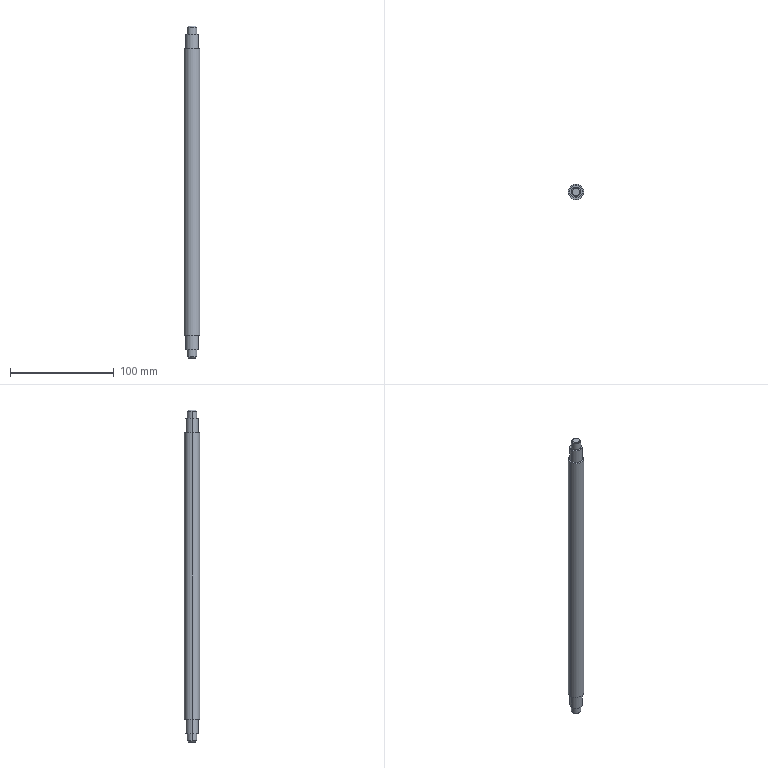Part | SolidWorks | features ICE 5, Chamfer 1, Extrusion 1, MirrorPattern 1 | 1 solid | 20 faces | box 15 x 15 x 320 mm | volume 52932 mm3 | cylinder 10 | plane 6 | cone 4 | commonest cylinder face diameters 9 x4 12 x4 15 x2
STEP:
#1=CARTESIAN_POINT('',(-3.5,0.,0.));
#2=VERTEX_POINT('',#1);
#3=CARTESIAN_POINT('',(3.5,0.,0.));
#4=VERTEX_POINT('',#3);
#5=CARTESIAN_POINT('',(0.,0.,0.));
#6=DIRECTION('',(0.,0.,-1.));
#7=DIRECTION('',(1.,0.,0.));
#8=AXIS2_PLACEMENT_3D('',#5,#6,#7);
#9=CIRCLE('',#8,3.5);
#10=EDGE_CURVE('',#2,#4,#9,.T.);
#11=ORIENTED_EDGE('',*,*,#10,.F.);
#12=CARTESIAN_POINT('',(-4.5,0.,1.));
#13=VERTEX_POINT('',#12);
#14=CARTESIAN_POINT('',(-4.5,0.,1.));
#15=DIRECTION('',(-0.7071,0.,0.7071));
#16=VECTOR('',#15,1000.);
#17=LINE('',#14,#16);
#18=EDGE_CURVE('',#2,#13,#17,.T.);
#19=ORIENTED_EDGE('',*,*,#18,.T.);
#20=CARTESIAN_POINT('',(4.5,0.,1.));
#21=VERTEX_POINT('',#20);
#22=CARTESIAN_POINT('',(0.,0.,1.));
#23=DIRECTION('',(0.,0.,1.));
#24=DIRECTION('',(1.,0.,0.));
#25=AXIS2_PLACEMENT_3D('',#22,#23,#24);
#26=CIRCLE('',#25,4.5);
#27=EDGE_CURVE('',#21,#13,#26,.T.);
#28=ORIENTED_EDGE('',*,*,#27,.F.);
#29=CARTESIAN_POINT('',(4.5,0.,1.));
#30=DIRECTION('',(0.7071,0.,0.7071));
#31=VECTOR('',#30,1000.);
#32=LINE('',#29,#31);
#33=EDGE_CURVE('',#4,#21,#32,.T.);
#34=ORIENTED_EDGE('',*,*,#33,.F.);
#35=EDGE_LOOP('',(#11,#19,#28,#34));
#36=FACE_OUTER_BOUND('',#35,.T.);
#37=CARTESIAN_POINT('',(0.,0.,1.));
#38=DIRECTION('',(0.,0.,1.));
#39=DIRECTION('',(1.,0.,0.));
#40=AXIS2_PLACEMENT_3D('',#37,#38,#39);
#41=CONICAL_SURFACE('',#40,4.5,0.7854);
#42=ADVANCED_FACE('',(#36),#41,.T.);
#43=CARTESIAN_POINT('',(3.5,0.,320.));
#44=VERTEX_POINT('',#43);
#45=CARTESIAN_POINT('',(-3.5,0.,320.));
#46=VERTEX_POINT('',#45);
#47=CARTESIAN_POINT('',(0.,0.,320.));
#48=DIRECTION('',(0.,0.,1.));
#49=DIRECTION('',(1.,0.,0.));
#50=AXIS2_PLACEMENT_3D('',#47,#48,#49);
#51=CIRCLE('',#50,3.5);
#52=EDGE_CURVE('',#44,#46,#51,.T.);
#53=ORIENTED_EDGE('',*,*,#52,.F.);
#54=CARTESIAN_POINT('',(4.5,0.,319.));
#55=VERTEX_POINT('',#54);
#56=CARTESIAN_POINT('',(3.5,0.,320.));
#57=DIRECTION('',(0.7071,0.,-0.7071));
#58=VECTOR('',#57,1000.);
#59=LINE('',#56,#58);
#60=EDGE_CURVE('',#44,#55,#59,.T.);
#61=ORIENTED_EDGE('',*,*,#60,.T.);
#62=CARTESIAN_POINT('',(-4.5,0.,319.));
#63=VERTEX_POINT('',#62);
#64=CARTESIAN_POINT('',(0.,0.,319.));
#65=DIRECTION('',(0.,0.,-1.));
#66=DIRECTION('',(1.,0.,0.));
#67=AXIS2_PLACEMENT_3D('',#64,#65,#66);
#68=CIRCLE('',#67,4.5);
#69=EDGE_CURVE('',#63,#55,#68,.T.);
#70=ORIENTED_EDGE('',*,*,#69,.F.);
#71=CARTESIAN_POINT('',(-3.5,0.,320.));
#72=DIRECTION('',(-0.7071,0.,-0.7071));
#73=VECTOR('',#72,1000.);
#74=LINE('',#71,#73);
#75=EDGE_CURVE('',#46,#63,#74,.T.);
#76=ORIENTED_EDGE('',*,*,#75,.F.);
#77=EDGE_LOOP('',(#53,#61,#70,#76));
#78=FACE_OUTER_BOUND('',#77,.T.);
#79=CARTESIAN_POINT('',(0.,0.,320.));
#80=DIRECTION('',(0.,0.,-1.));
#81=DIRECTION('',(-1.,0.,0.));
#82=AXIS2_PLACEMENT_3D('',#79,#80,#81);
#83=CONICAL_SURFACE('',#82,3.5,0.7854);
#84=ADVANCED_FACE('',(#78),#83,.T.);
#85=ORIENTED_EDGE('',*,*,#69,.T.);
#86=CARTESIAN_POINT('',(4.5,0.,312.));
#87=VERTEX_POINT('',#86);
#88=CARTESIAN_POINT('',(4.5,0.,320.));
#89=DIRECTION('',(0.,0.,-1.));
#90=VECTOR('',#89,1000.);
#91=LINE('',#88,#90);
#92=EDGE_CURVE('',#55,#87,#91,.T.);
#93=ORIENTED_EDGE('',*,*,#92,.T.);
#94=CARTESIAN_POINT('',(-4.5,0.,312.));
#95=VERTEX_POINT('',#94);
#96=CARTESIAN_POINT('',(0.,0.,312.));
#97=DIRECTION('',(0.,0.,1.));
#98=DIRECTION('',(1.,0.,0.));
#99=AXIS2_PLACEMENT_3D('',#96,#97,#98);
#100=CIRCLE('',#99,4.5);
#101=EDGE_CURVE('',#87,#95,#100,.T.);
#102=ORIENTED_EDGE('',*,*,#101,.T.);
#103=CARTESIAN_POINT('',(-4.5,0.,320.));
#104=DIRECTION('',(0.,0.,-1.));
#105=VECTOR('',#104,1000.);
#106=LINE('',#103,#105);
#107=EDGE_CURVE('',#63,#95,#106,.T.);
#108=ORIENTED_EDGE('',*,*,#107,.F.);
#109=EDGE_LOOP('',(#85,#93,#102,#108));
#110=FACE_OUTER_BOUND('',#109,.T.);
#111=CARTESIAN_POINT('',(0.,0.,320.));
#112=DIRECTION('',(0.,0.,-1.));
#113=DIRECTION('',(-1.,0.,0.));
#114=AXIS2_PLACEMENT_3D('',#111,#112,#113);
#115=CYLINDRICAL_SURFACE('',#114,4.5);
#116=ADVANCED_FACE('',(#110),#115,.T.);
#117=CARTESIAN_POINT('',(6.,0.,312.));
#118=VERTEX_POINT('',#117);
#119=CARTESIAN_POINT('',(-6.,0.,312.));
#120=VERTEX_POINT('',#119);
#121=CARTESIAN_POINT('',(0.,0.,312.));
#122=DIRECTION('',(0.,0.,1.));
#123=DIRECTION('',(1.,0.,0.));
#124=AXIS2_PLACEMENT_3D('',#121,#122,#123);
#125=CIRCLE('',#124,6.);
#126=EDGE_CURVE('',#118,#120,#125,.T.);
#127=ORIENTED_EDGE('',*,*,#126,.F.);
#128=CARTESIAN_POINT('',(6.,0.,298.));
#129=VERTEX_POINT('',#128);
#130=CARTESIAN_POINT('',(6.,0.,312.));
#131=DIRECTION('',(0.,0.,-1.));
#132=VECTOR('',#131,1000.);
#133=LINE('',#130,#132);
#134=EDGE_CURVE('',#118,#129,#133,.T.);
#135=ORIENTED_EDGE('',*,*,#134,.T.);
#136=CARTESIAN_POINT('',(-6.,0.,298.));
#137=VERTEX_POINT('',#136);
#138=CARTESIAN_POINT('',(0.,0.,298.));
#139=DIRECTION('',(0.,0.,1.));
#140=DIRECTION('',(1.,0.,0.));
#141=AXIS2_PLACEMENT_3D('',#138,#139,#140);
#142=CIRCLE('',#141,6.);
#143=EDGE_CURVE('',#129,#137,#142,.T.);
#144=ORIENTED_EDGE('',*,*,#143,.T.);
#145=CARTESIAN_POINT('',(-6.,0.,312.));
#146=DIRECTION('',(0.,0.,-1.));
#147=VECTOR('',#146,1000.);
#148=LINE('',#145,#147);
#149=EDGE_CURVE('',#120,#137,#148,.T.);
#150=ORIENTED_EDGE('',*,*,#149,.F.);
#151=EDGE_LOOP('',(#127,#135,#144,#150));
#152=FACE_OUTER_BOUND('',#151,.T.);
#153=CARTESIAN_POINT('',(0.,0.,312.));
#154=DIRECTION('',(0.,0.,-1.));
#155=DIRECTION('',(-1.,0.,0.));
#156=AXIS2_PLACEMENT_3D('',#153,#154,#155);
#157=CYLINDRICAL_SURFACE('',#156,6.);
#158=ADVANCED_FACE('',(#152),#157,.T.);
#159=CARTESIAN_POINT('',(7.5,0.,298.));
#160=VERTEX_POINT('',#159);
#161=CARTESIAN_POINT('',(-7.5,0.,298.));
#162=VERTEX_POINT('',#161);
#163=CARTESIAN_POINT('',(0.,0.,298.));
#164=DIRECTION('',(0.,0.,1.));
#165=DIRECTION('',(1.,0.,0.));
#166=AXIS2_PLACEMENT_3D('',#163,#164,#165);
#167=CIRCLE('',#166,7.5);
#168=EDGE_CURVE('',#160,#162,#167,.T.);
#169=ORIENTED_EDGE('',*,*,#168,.F.);
#170=CARTESIAN_POINT('',(7.5,0.,22.));
#171=VERTEX_POINT('',#170);
#172=CARTESIAN_POINT('',(7.5,0.,298.));
#173=DIRECTION('',(0.,0.,-1.));
#174=VECTOR('',#173,1000.);
#175=LINE('',#172,#174);
#176=EDGE_CURVE('',#160,#171,#175,.T.);
#177=ORIENTED_EDGE('',*,*,#176,.T.);
#178=CARTESIAN_POINT('',(-7.5,0.,22.));
#179=VERTEX_POINT('',#178);
#180=CARTESIAN_POINT('',(0.,0.,22.));
#181=DIRECTION('',(0.,0.,1.));
#182=DIRECTION('',(1.,0.,0.));
#183=AXIS2_PLACEMENT_3D('',#180,#181,#182);
#184=CIRCLE('',#183,7.5);
#185=EDGE_CURVE('',#171,#179,#184,.T.);
#186=ORIENTED_EDGE('',*,*,#185,.T.);
#187=CARTESIAN_POINT('',(-7.5,0.,298.));
#188=DIRECTION('',(0.,0.,-1.));
#189=VECTOR('',#188,1000.);
#190=LINE('',#187,#189);
#191=EDGE_CURVE('',#162,#179,#190,.T.);
#192=ORIENTED_EDGE('',*,*,#191,.F.);
#193=EDGE_LOOP('',(#169,#177,#186,#192));
#194=FACE_OUTER_BOUND('',#193,.T.);
#195=CARTESIAN_POINT('',(0.,0.,298.));
#196=DIRECTION('',(0.,0.,-1.));
#197=DIRECTION('',(-1.,0.,0.));
#198=AXIS2_PLACEMENT_3D('',#195,#196,#197);
#199=CYLINDRICAL_SURFACE('',#198,7.5);
#200=ADVANCED_FACE('',(#194),#199,.T.);
#201=CARTESIAN_POINT('',(6.,0.,22.));
#202=VERTEX_POINT('',#201);
#203=CARTESIAN_POINT('',(-6.,0.,22.));
#204=VERTEX_POINT('',#203);
#205=CARTESIAN_POINT('',(0.,0.,22.));
#206=DIRECTION('',(0.,0.,1.));
#207=DIRECTION('',(1.,0.,0.));
#208=AXIS2_PLACEMENT_3D('',#205,#206,#207);
#209=CIRCLE('',#208,6.);
#210=EDGE_CURVE('',#202,#204,#209,.T.);
#211=ORIENTED_EDGE('',*,*,#210,.F.);
#212=CARTESIAN_POINT('',(6.,0.,8.));
#213=VERTEX_POINT('',#212);
#214=CARTESIAN_POINT('',(6.,0.,22.));
#215=DIRECTION('',(0.,0.,-1.));
#216=VECTOR('',#215,1000.);
#217=LINE('',#214,#216);
#218=EDGE_CURVE('',#202,#213,#217,.T.);
#219=ORIENTED_EDGE('',*,*,#218,.T.);
#220=CARTESIAN_POINT('',(-6.,0.,8.));
#221=VERTEX_POINT('',#220);
#222=CARTESIAN_POINT('',(0.,0.,8.));
#223=DIRECTION('',(0.,0.,1.));
#224=DIRECTION('',(1.,0.,0.));
#225=AXIS2_PLACEMENT_3D('',#222,#223,#224);
#226=CIRCLE('',#225,6.);
#227=EDGE_CURVE('',#213,#221,#226,.T.);
#228=ORIENTED_EDGE('',*,*,#227,.T.);
#229=CARTESIAN_POINT('',(-6.,0.,22.));
#230=DIRECTION('',(0.,0.,-1.));
#231=VECTOR('',#230,1000.);
#232=LINE('',#229,#231);
#233=EDGE_CURVE('',#204,#221,#232,.T.);
#234=ORIENTED_EDGE('',*,*,#233,.F.);
#235=EDGE_LOOP('',(#211,#219,#228,#234));
#236=FACE_OUTER_BOUND('',#235,.T.);
#237=CARTESIAN_POINT('',(0.,0.,22.));
#238=DIRECTION('',(0.,0.,-1.));
#239=DIRECTION('',(-1.,0.,0.));
#240=AXIS2_PLACEMENT_3D('',#237,#238,#239);
#241=CYLINDRICAL_SURFACE('',#240,6.);
#242=ADVANCED_FACE('',(#236),#241,.T.);
#243=CARTESIAN_POINT('',(4.5,0.,8.));
#244=VERTEX_POINT('',#243);
#245=CARTESIAN_POINT('',(-4.5,0.,8.));
#246=VERTEX_POINT('',#245);
#247=CARTESIAN_POINT('',(0.,0.,8.));
#248=DIRECTION('',(0.,0.,1.));
#249=DIRECTION('',(1.,0.,0.));
#250=AXIS2_PLACEMENT_3D('',#247,#248,#249);
#251=CIRCLE('',#250,4.5);
#252=EDGE_CURVE('',#244,#246,#251,.T.);
#253=ORIENTED_EDGE('',*,*,#252,.F.);
#254=CARTESIAN_POINT('',(4.5,0.,8.));
#255=DIRECTION('',(0.,0.,-1.));
#256=VECTOR('',#255,1000.);
#257=LINE('',#254,#256);
#258=EDGE_CURVE('',#244,#21,#257,.T.);
#259=ORIENTED_EDGE('',*,*,#258,.T.);
#260=ORIENTED_EDGE('',*,*,#27,.T.);
#261=CARTESIAN_POINT('',(-4.5,0.,8.));
#262=DIRECTION('',(0.,0.,-1.));
#263=VECTOR('',#262,1000.);
#264=LINE('',#261,#263);
#265=EDGE_CURVE('',#246,#13,#264,.T.);
#266=ORIENTED_EDGE('',*,*,#265,.F.);
#267=EDGE_LOOP('',(#253,#259,#260,#266));
#268=FACE_OUTER_BOUND('',#267,.T.);
#269=CARTESIAN_POINT('',(0.,0.,8.));
#270=DIRECTION('',(0.,0.,-1.));
#271=DIRECTION('',(-1.,0.,0.));
#272=AXIS2_PLACEMENT_3D('',#269,#270,#271);
#273=CYLINDRICAL_SURFACE('',#272,4.5);
#274=ADVANCED_FACE('',(#268),#273,.T.);
#275=ORIENTED_EDGE('',*,*,#258,.F.);
#276=CARTESIAN_POINT('',(0.,0.,8.));
#277=DIRECTION('',(0.,0.,1.));
#278=DIRECTION('',(1.,0.,0.));
#279=AXIS2_PLACEMENT_3D('',#276,#277,#278);
#280=CIRCLE('',#279,4.5);
#281=EDGE_CURVE('',#246,#244,#280,.T.);
#282=ORIENTED_EDGE('',*,*,#281,.F.);
#283=ORIENTED_EDGE('',*,*,#265,.T.);
#284=CARTESIAN_POINT('',(0.,0.,1.));
#285=DIRECTION('',(0.,0.,1.));
#286=DIRECTION('',(1.,0.,0.));
#287=AXIS2_PLACEMENT_3D('',#284,#285,#286);
#288=CIRCLE('',#287,4.5);
#289=EDGE_CURVE('',#13,#21,#288,.T.);
#290=ORIENTED_EDGE('',*,*,#289,.T.);
#291=EDGE_LOOP('',(#275,#282,#283,#290));
#292=FACE_OUTER_BOUND('',#291,.T.);
#293=CARTESIAN_POINT('',(0.,0.,8.));
#294=DIRECTION('',(0.,0.,-1.));
#295=DIRECTION('',(-1.,0.,0.));
#296=AXIS2_PLACEMENT_3D('',#293,#294,#295);
#297=CYLINDRICAL_SURFACE('',#296,4.5);
#298=ADVANCED_FACE('',(#292),#297,.T.);
#299=CARTESIAN_POINT('',(0.,0.,0.));
#300=DIRECTION('',(0.,0.,-1.));
#301=DIRECTION('',(1.,0.,0.));
#302=AXIS2_PLACEMENT_3D('',#299,#300,#301);
#303=CIRCLE('',#302,3.5);
#304=EDGE_CURVE('',#4,#2,#303,.T.);
#305=ORIENTED_EDGE('',*,*,#304,.T.);
#306=ORIENTED_EDGE('',*,*,#10,.T.);
#307=EDGE_LOOP('',(#305,#306));
#308=FACE_OUTER_BOUND('',#307,.T.);
#309=CARTESIAN_POINT('',(0.,0.,0.));
#310=DIRECTION('',(0.,0.,1.));
#311=DIRECTION('',(1.,0.,0.));
#312=AXIS2_PLACEMENT_3D('',#309,#310,#311);
#313=PLANE('',#312);
#314=ADVANCED_FACE('',(#308),#313,.F.);
#315=ORIENTED_EDGE('',*,*,#218,.F.);
#316=CARTESIAN_POINT('',(0.,0.,22.));
#317=DIRECTION('',(0.,0.,1.));
#318=DIRECTION('',(1.,0.,0.));
#319=AXIS2_PLACEMENT_3D('',#316,#317,#318);
#320=CIRCLE('',#319,6.);
#321=EDGE_CURVE('',#204,#202,#320,.T.);
#322=ORIENTED_EDGE('',*,*,#321,.F.);
#323=ORIENTED_EDGE('',*,*,#233,.T.);
#324=CARTESIAN_POINT('',(0.,0.,8.));
#325=DIRECTION('',(0.,0.,1.));
#326=DIRECTION('',(1.,0.,0.));
#327=AXIS2_PLACEMENT_3D('',#324,#325,#326);
#328=CIRCLE('',#327,6.);
#329=EDGE_CURVE('',#221,#213,#328,.T.);
#330=ORIENTED_EDGE('',*,*,#329,.T.);
#331=EDGE_LOOP('',(#315,#322,#323,#330));
#332=FACE_OUTER_BOUND('',#331,.T.);
#333=CARTESIAN_POINT('',(0.,0.,22.));
#334=DIRECTION('',(0.,0.,-1.));
#335=DIRECTION('',(-1.,0.,0.));
#336=AXIS2_PLACEMENT_3D('',#333,#334,#335);
#337=CYLINDRICAL_SURFACE('',#336,6.);
#338=ADVANCED_FACE('',(#332),#337,.T.);
#339=ORIENTED_EDGE('',*,*,#281,.T.);
#340=ORIENTED_EDGE('',*,*,#252,.T.);
#341=EDGE_LOOP('',(#339,#340));
#342=FACE_BOUND('',#341,.T.);
#343=ORIENTED_EDGE('',*,*,#329,.F.);
#344=ORIENTED_EDGE('',*,*,#227,.F.);
#345=EDGE_LOOP('',(#343,#344));
#346=FACE_OUTER_BOUND('',#345,.T.);
#347=CARTESIAN_POINT('',(0.,0.,8.));
#348=DIRECTION('',(0.,0.,1.));
#349=DIRECTION('',(1.,0.,0.));
#350=AXIS2_PLACEMENT_3D('',#347,#348,#349);
#351=PLANE('',#350);
#352=ADVANCED_FACE('',(#342,#346),#351,.F.);
#353=ORIENTED_EDGE('',*,*,#176,.F.);
#354=CARTESIAN_POINT('',(0.,0.,298.));
#355=DIRECTION('',(0.,0.,1.));
#356=DIRECTION('',(1.,0.,0.));
#357=AXIS2_PLACEMENT_3D('',#354,#355,#356);
#358=CIRCLE('',#357,7.5);
#359=EDGE_CURVE('',#162,#160,#358,.T.);
#360=ORIENTED_EDGE('',*,*,#359,.F.);
#361=ORIENTED_EDGE('',*,*,#191,.T.);
#362=CARTESIAN_POINT('',(0.,0.,22.));
#363=DIRECTION('',(0.,0.,1.));
#364=DIRECTION('',(1.,0.,0.));
#365=AXIS2_PLACEMENT_3D('',#362,#363,#364);
#366=CIRCLE('',#365,7.5);
#367=EDGE_CURVE('',#179,#171,#366,.T.);
#368=ORIENTED_EDGE('',*,*,#367,.T.);
#369=EDGE_LOOP('',(#353,#360,#361,#368));
#370=FACE_OUTER_BOUND('',#369,.T.);
#371=CARTESIAN_POINT('',(0.,0.,298.));
#372=DIRECTION('',(0.,0.,-1.));
#373=DIRECTION('',(-1.,0.,0.));
#374=AXIS2_PLACEMENT_3D('',#371,#372,#373);
#375=CYLINDRICAL_SURFACE('',#374,7.5);
#376=ADVANCED_FACE('',(#370),#375,.T.);
#377=CARTESIAN_POINT('',(0.,0.,298.));
#378=DIRECTION('',(0.,0.,1.));
#379=DIRECTION('',(1.,0.,0.));
#380=AXIS2_PLACEMENT_3D('',#377,#378,#379);
#381=CIRCLE('',#380,6.);
#382=EDGE_CURVE('',#137,#129,#381,.T.);
#383=ORIENTED_EDGE('',*,*,#382,.F.);
#384=ORIENTED_EDGE('',*,*,#143,.F.);
#385=EDGE_LOOP('',(#383,#384));
#386=FACE_BOUND('',#385,.T.);
#387=ORIENTED_EDGE('',*,*,#359,.T.);
#388=ORIENTED_EDGE('',*,*,#168,.T.);
#389=EDGE_LOOP('',(#387,#388));
#390=FACE_OUTER_BOUND('',#389,.T.);
#391=CARTESIAN_POINT('',(0.,0.,298.));
#392=DIRECTION('',(0.,0.,1.));
#393=DIRECTION('',(1.,0.,0.));
#394=AXIS2_PLACEMENT_3D('',#391,#392,#393);
#395=PLANE('',#394);
#396=ADVANCED_FACE('',(#386,#390),#395,.T.);
#397=ORIENTED_EDGE('',*,*,#321,.T.);
#398=ORIENTED_EDGE('',*,*,#210,.T.);
#399=EDGE_LOOP('',(#397,#398));
#400=FACE_BOUND('',#399,.T.);
#401=ORIENTED_EDGE('',*,*,#367,.F.);
#402=ORIENTED_EDGE('',*,*,#185,.F.);
#403=EDGE_LOOP('',(#401,#402));
#404=FACE_OUTER_BOUND('',#403,.T.);
#405=CARTESIAN_POINT('',(0.,0.,22.));
#406=DIRECTION('',(0.,0.,1.));
#407=DIRECTION('',(1.,0.,0.));
#408=AXIS2_PLACEMENT_3D('',#405,#406,#407);
#409=PLANE('',#408);
#410=ADVANCED_FACE('',(#400,#404),#409,.F.);
#411=ORIENTED_EDGE('',*,*,#134,.F.);
#412=CARTESIAN_POINT('',(0.,0.,312.));
#413=DIRECTION('',(0.,0.,1.));
#414=DIRECTION('',(1.,0.,0.));
#415=AXIS2_PLACEMENT_3D('',#412,#413,#414);
#416=CIRCLE('',#415,6.);
#417=EDGE_CURVE('',#120,#118,#416,.T.);
#418=ORIENTED_EDGE('',*,*,#417,.F.);
#419=ORIENTED_EDGE('',*,*,#149,.T.);
#420=ORIENTED_EDGE('',*,*,#382,.T.);
#421=EDGE_LOOP('',(#411,#418,#419,#420));
#422=FACE_OUTER_BOUND('',#421,.T.);
#423=CARTESIAN_POINT('',(0.,0.,312.));
#424=DIRECTION('',(0.,0.,-1.));
#425=DIRECTION('',(-1.,0.,0.));
#426=AXIS2_PLACEMENT_3D('',#423,#424,#425);
#427=CYLINDRICAL_SURFACE('',#426,6.);
#428=ADVANCED_FACE('',(#422),#427,.T.);
#429=CARTESIAN_POINT('',(0.,0.,312.));
#430=DIRECTION('',(0.,0.,1.));
#431=DIRECTION('',(1.,0.,0.));
#432=AXIS2_PLACEMENT_3D('',#429,#430,#431);
#433=CIRCLE('',#432,4.5);
#434=EDGE_CURVE('',#95,#87,#433,.T.);
#435=ORIENTED_EDGE('',*,*,#434,.F.);
#436=ORIENTED_EDGE('',*,*,#101,.F.);
#437=EDGE_LOOP('',(#435,#436));
#438=FACE_BOUND('',#437,.T.);
#439=ORIENTED_EDGE('',*,*,#417,.T.);
#440=ORIENTED_EDGE('',*,*,#126,.T.);
#441=EDGE_LOOP('',(#439,#440));
#442=FACE_OUTER_BOUND('',#441,.T.);
#443=CARTESIAN_POINT('',(0.,0.,312.));
#444=DIRECTION('',(0.,0.,1.));
#445=DIRECTION('',(1.,0.,0.));
#446=AXIS2_PLACEMENT_3D('',#443,#444,#445);
#447=PLANE('',#446);
#448=ADVANCED_FACE('',(#438,#442),#447,.T.);
#449=ORIENTED_EDGE('',*,*,#92,.F.);
#450=CARTESIAN_POINT('',(0.,0.,319.));
#451=DIRECTION('',(0.,0.,-1.));
#452=DIRECTION('',(1.,0.,0.));
#453=AXIS2_PLACEMENT_3D('',#450,#451,#452);
#454=CIRCLE('',#453,4.5);
#455=EDGE_CURVE('',#55,#63,#454,.T.);
#456=ORIENTED_EDGE('',*,*,#455,.T.);
#457=ORIENTED_EDGE('',*,*,#107,.T.);
#458=ORIENTED_EDGE('',*,*,#434,.T.);
#459=EDGE_LOOP('',(#449,#456,#457,#458));
#460=FACE_OUTER_BOUND('',#459,.T.);
#461=CARTESIAN_POINT('',(0.,0.,320.));
#462=DIRECTION('',(0.,0.,-1.));
#463=DIRECTION('',(-1.,0.,0.));
#464=AXIS2_PLACEMENT_3D('',#461,#462,#463);
#465=CYLINDRICAL_SURFACE('',#464,4.5);
#466=ADVANCED_FACE('',(#460),#465,.T.);
#467=CARTESIAN_POINT('',(0.,0.,320.));
#468=DIRECTION('',(0.,0.,1.));
#469=DIRECTION('',(1.,0.,0.));
#470=AXIS2_PLACEMENT_3D('',#467,#468,#469);
#471=CIRCLE('',#470,3.5);
#472=EDGE_CURVE('',#46,#44,#471,.T.);
#473=ORIENTED_EDGE('',*,*,#472,.T.);
#474=ORIENTED_EDGE('',*,*,#52,.T.);
#475=EDGE_LOOP('',(#473,#474));
#476=FACE_OUTER_BOUND('',#475,.T.);
#477=CARTESIAN_POINT('',(0.,0.,320.));
#478=DIRECTION('',(0.,0.,1.));
#479=DIRECTION('',(1.,0.,0.));
#480=AXIS2_PLACEMENT_3D('',#477,#478,#479);
#481=PLANE('',#480);
#482=ADVANCED_FACE('',(#476),#481,.T.);
#483=ORIENTED_EDGE('',*,*,#60,.F.);
#484=ORIENTED_EDGE('',*,*,#472,.F.);
#485=ORIENTED_EDGE('',*,*,#75,.T.);
#486=ORIENTED_EDGE('',*,*,#455,.F.);
#487=EDGE_LOOP('',(#483,#484,#485,#486));
#488=FACE_OUTER_BOUND('',#487,.T.);
#489=CARTESIAN_POINT('',(0.,0.,320.));
#490=DIRECTION('',(0.,0.,-1.));
#491=DIRECTION('',(-1.,0.,0.));
#492=AXIS2_PLACEMENT_3D('',#489,#490,#491);
#493=CONICAL_SURFACE('',#492,3.5,0.7854);
#494=ADVANCED_FACE('',(#488),#493,.T.);
#495=ORIENTED_EDGE('',*,*,#18,.F.);
#496=ORIENTED_EDGE('',*,*,#304,.F.);
#497=ORIENTED_EDGE('',*,*,#33,.T.);
#498=ORIENTED_EDGE('',*,*,#289,.F.);
#499=EDGE_LOOP('',(#495,#496,#497,#498));
#500=FACE_OUTER_BOUND('',#499,.T.);
#501=CARTESIAN_POINT('',(0.,0.,1.));
#502=DIRECTION('',(0.,0.,1.));
#503=DIRECTION('',(1.,0.,0.));
#504=AXIS2_PLACEMENT_3D('',#501,#502,#503);
#505=CONICAL_SURFACE('',#504,4.5,0.7854);
#506=ADVANCED_FACE('',(#500),#505,.T.);
#507=CLOSED_SHELL('',(#42,#84,#116,#158,#200,#242,#274,#298,#314,#338,#352,#376,#396,#410,#428,#448,#466,#482,#494,#506));
#508=MANIFOLD_SOLID_BREP('',#507);
#509=CARTESIAN_POINT('',(0.,0.,0.));
#510=DIRECTION('',(0.,0.,1.));
#511=DIRECTION('',(1.,0.,0.));
#512=AXIS2_PLACEMENT_3D('',#509,#510,#511);
#513=(LENGTH_UNIT()NAMED_UNIT(*)SI_UNIT(.MILLI.,.METRE.));
#514=UNCERTAINTY_MEASURE_WITH_UNIT(LENGTH_MEASURE(0.00001),#513,'','');
#515=(NAMED_UNIT(*)PLANE_ANGLE_UNIT()SI_UNIT($,.RADIAN.));
#516=(NAMED_UNIT(*)SI_UNIT($,.STERADIAN.)SOLID_ANGLE_UNIT());
#517=(GEOMETRIC_REPRESENTATION_CONTEXT(3)GLOBAL_UNCERTAINTY_ASSIGNED_CONTEXT((#514))GLOBAL_UNIT_ASSIGNED_CONTEXT((#513,#515,#516))REPRESENTATION_CONTEXT('',''));
#518=ADVANCED_BREP_SHAPE_REPRESENTATION('',(#508,#512),#517);